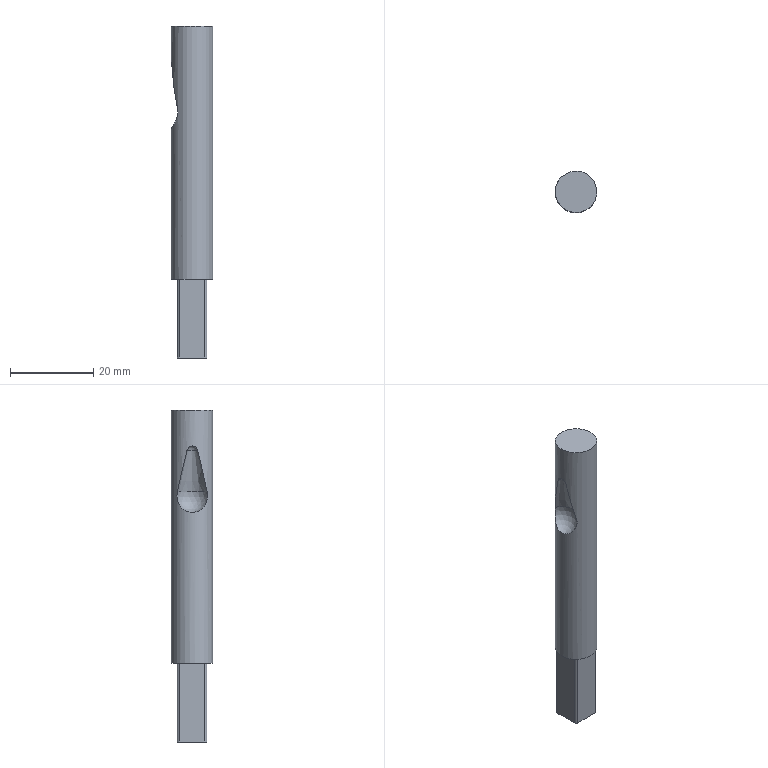Part | NX | features solid 2 | 1 solid | 15 faces | volume 5566 mm3 | plane 7 | cylinder 5 | sphere 2 | cone 1 | commonest cylinder face diameters 1.1 x4 10 x1